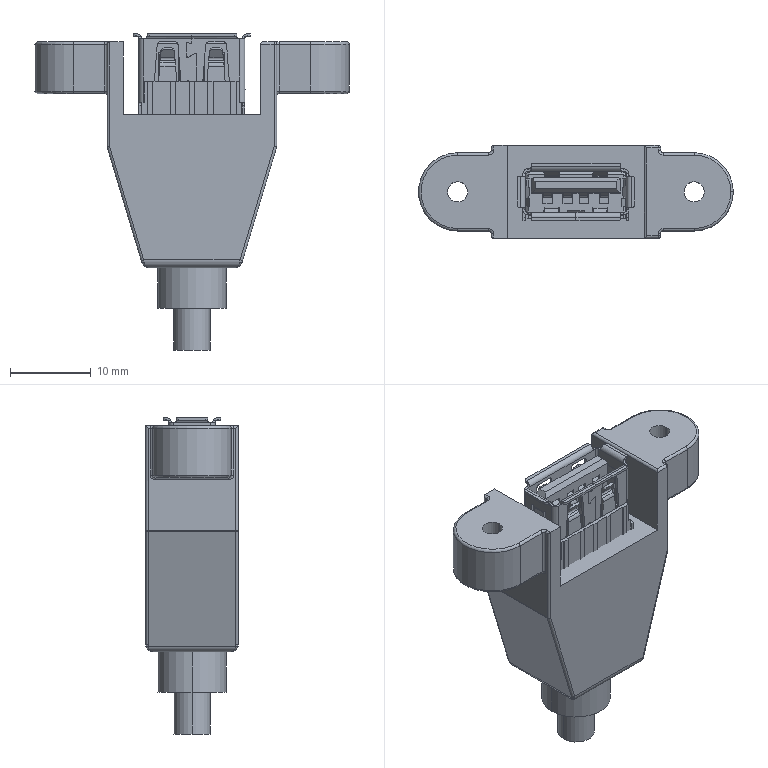Part | NX | features BREP 6 | 6 solids | 1052 faces | box 39 x 11.5 x 39.2 mm | volume 5931 mm3 | plane 635 | cylinder 345 | spline 50 | torus 14 | sphere 6 | cone 2 | commonest cylinder face diameters 0.6 x80 0.4 x59 1 x32 0.3 x24 1.2 x15 0.5 x12